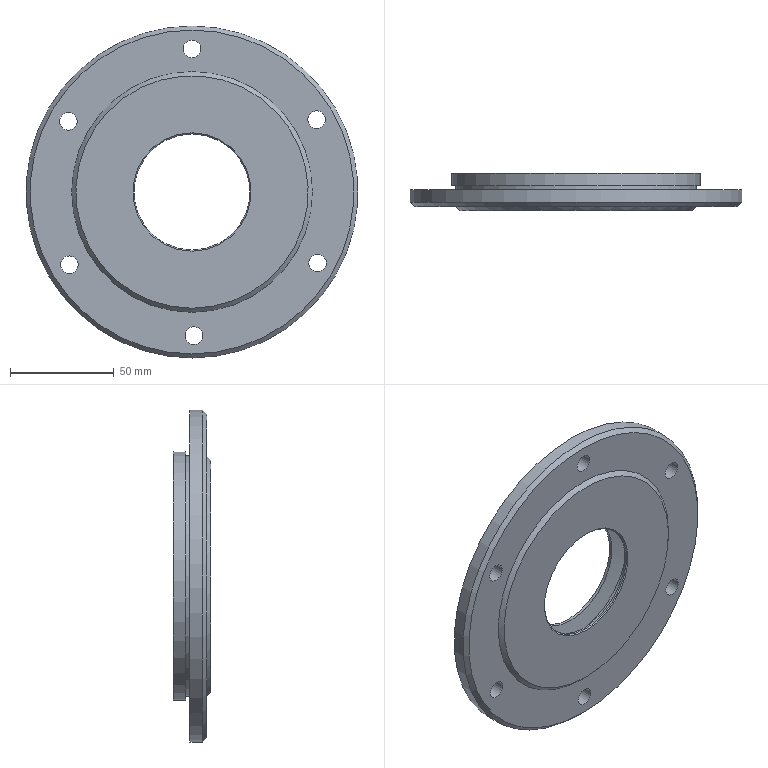Part | NX | features BREP 1, DATUM_CSYS 1 | 1 solid | 24 faces | box 160 x 18 x 160 mm | volume 177921 mm3 | cylinder 12 | plane 6 | cone 6 | commonest cylinder face diameters 8.5 x6 56 x2 74 x1 116 x1 120 x1 160 x1
STEP:
#1=CARTESIAN_POINT('',(419.528,84.,-38.494));
#2=VERTEX_POINT('',#1);
#3=CARTESIAN_POINT('',(419.528,84.,-34.244));
#4=DIRECTION('',(0.,-1.,0.));
#5=DIRECTION('',(0.,0.,-1.));
#6=AXIS2_PLACEMENT_3D('',#3,#4,#5);
#7=CIRCLE('',#6,4.25);
#8=EDGE_CURVE('',#2,#2,#7,.F.);
#9=ORIENTED_EDGE('',*,*,#8,.T.);
#10=EDGE_LOOP('',(#9));
#11=FACE_BOUND('',#10,.T.);
#12=CARTESIAN_POINT('',(359.92,84.,-73.44));
#13=VERTEX_POINT('',#12);
#14=CARTESIAN_POINT('',(359.92,84.,-69.19));
#15=DIRECTION('',(0.,-1.,0.));
#16=DIRECTION('',(0.,0.,-1.));
#17=AXIS2_PLACEMENT_3D('',#14,#15,#16);
#18=CIRCLE('',#17,4.25);
#19=EDGE_CURVE('',#13,#13,#18,.F.);
#20=ORIENTED_EDGE('',*,*,#19,.T.);
#21=EDGE_LOOP('',(#20));
#22=FACE_BOUND('',#21,.T.);
#23=CARTESIAN_POINT('',(299.852,84.,-39.291));
#24=VERTEX_POINT('',#23);
#25=CARTESIAN_POINT('',(299.852,84.,-35.041));
#26=DIRECTION('',(0.,-1.,0.));
#27=DIRECTION('',(0.,0.,-1.));
#28=AXIS2_PLACEMENT_3D('',#25,#26,#27);
#29=CIRCLE('',#28,4.25);
#30=EDGE_CURVE('',#24,#24,#29,.F.);
#31=ORIENTED_EDGE('',*,*,#30,.T.);
#32=EDGE_LOOP('',(#31));
#33=FACE_BOUND('',#32,.T.);
#34=CARTESIAN_POINT('',(299.392,84.,29.804));
#35=VERTEX_POINT('',#34);
#36=CARTESIAN_POINT('',(299.392,84.,34.054));
#37=DIRECTION('',(0.,-1.,0.));
#38=DIRECTION('',(0.,0.,-1.));
#39=AXIS2_PLACEMENT_3D('',#36,#37,#38);
#40=CIRCLE('',#39,4.25);
#41=EDGE_CURVE('',#35,#35,#40,.F.);
#42=ORIENTED_EDGE('',*,*,#41,.T.);
#43=EDGE_LOOP('',(#42));
#44=FACE_BOUND('',#43,.T.);
#45=CARTESIAN_POINT('',(359.,84.,64.75));
#46=VERTEX_POINT('',#45);
#47=CARTESIAN_POINT('',(359.,84.,69.));
#48=DIRECTION('',(0.,-1.,0.));
#49=DIRECTION('',(0.,0.,-1.));
#50=AXIS2_PLACEMENT_3D('',#47,#48,#49);
#51=CIRCLE('',#50,4.25);
#52=EDGE_CURVE('',#46,#46,#51,.F.);
#53=ORIENTED_EDGE('',*,*,#52,.T.);
#54=EDGE_LOOP('',(#53));
#55=FACE_BOUND('',#54,.T.);
#56=CARTESIAN_POINT('',(419.068,84.,30.601));
#57=VERTEX_POINT('',#56);
#58=CARTESIAN_POINT('',(419.068,84.,34.851));
#59=DIRECTION('',(0.,-1.,0.));
#60=DIRECTION('',(0.,0.,-1.));
#61=AXIS2_PLACEMENT_3D('',#58,#59,#60);
#62=CIRCLE('',#61,4.25);
#63=EDGE_CURVE('',#57,#57,#62,.F.);
#64=ORIENTED_EDGE('',*,*,#63,.T.);
#65=EDGE_LOOP('',(#64));
#66=FACE_BOUND('',#65,.T.);
#67=CARTESIAN_POINT('',(359.,84.,-78.));
#68=VERTEX_POINT('',#67);
#69=CARTESIAN_POINT('',(359.,84.,0.));
#70=DIRECTION('',(0.,-1.,0.));
#71=DIRECTION('',(0.,0.,-1.));
#72=AXIS2_PLACEMENT_3D('',#69,#70,#71);
#73=CIRCLE('',#72,78.);
#74=EDGE_CURVE('',#68,#68,#73,.T.);
#75=ORIENTED_EDGE('',*,*,#74,.T.);
#76=EDGE_LOOP('',(#75));
#77=FACE_BOUND('',#76,.T.);
#78=CARTESIAN_POINT('',(359.,84.,-58.));
#79=VERTEX_POINT('',#78);
#80=CARTESIAN_POINT('',(359.,84.,0.));
#81=DIRECTION('',(0.,-1.,0.));
#82=DIRECTION('',(0.,0.,-1.));
#83=AXIS2_PLACEMENT_3D('',#80,#81,#82);
#84=CIRCLE('',#83,58.);
#85=EDGE_CURVE('',#79,#79,#84,.T.);
#86=ORIENTED_EDGE('',*,*,#85,.F.);
#87=EDGE_LOOP('',(#86));
#88=FACE_BOUND('',#87,.T.);
#89=CARTESIAN_POINT('',(417.,84.,0.));
#90=DIRECTION('',(0.,-1.,0.));
#91=DIRECTION('',(0.,0.,-1.));
#92=AXIS2_PLACEMENT_3D('',#89,#90,#91);
#93=PLANE('',#92);
#94=ADVANCED_FACE('',(#11,#22,#33,#44,#55,#66,#77,#88),#93,.T.);
#95=CARTESIAN_POINT('',(359.,86.,-80.));
#96=VERTEX_POINT('',#95);
#97=CARTESIAN_POINT('',(359.,86.,0.));
#98=DIRECTION('',(0.,-1.,0.));
#99=DIRECTION('',(0.,0.,-1.));
#100=AXIS2_PLACEMENT_3D('',#97,#98,#99);
#101=CIRCLE('',#100,80.);
#102=EDGE_CURVE('',#96,#96,#101,.T.);
#103=ORIENTED_EDGE('',*,*,#102,.T.);
#104=EDGE_LOOP('',(#103));
#105=FACE_BOUND('',#104,.T.);
#106=ORIENTED_EDGE('',*,*,#74,.F.);
#107=EDGE_LOOP('',(#106));
#108=FACE_BOUND('',#107,.T.);
#109=CARTESIAN_POINT('',(359.,84.,0.));
#110=DIRECTION('',(0.,1.,0.));
#111=DIRECTION('',(0.,0.,1.));
#112=AXIS2_PLACEMENT_3D('',#109,#110,#111);
#113=CONICAL_SURFACE('',#112,78.,0.7854);
#114=ADVANCED_FACE('',(#105,#108),#113,.T.);
#115=CARTESIAN_POINT('',(359.,92.,-80.));
#116=VERTEX_POINT('',#115);
#117=CARTESIAN_POINT('',(359.,92.,0.));
#118=DIRECTION('',(0.,-1.,0.));
#119=DIRECTION('',(0.,0.,-1.));
#120=AXIS2_PLACEMENT_3D('',#117,#118,#119);
#121=CIRCLE('',#120,80.);
#122=EDGE_CURVE('',#116,#116,#121,.T.);
#123=ORIENTED_EDGE('',*,*,#122,.T.);
#124=EDGE_LOOP('',(#123));
#125=FACE_BOUND('',#124,.T.);
#126=ORIENTED_EDGE('',*,*,#102,.F.);
#127=EDGE_LOOP('',(#126));
#128=FACE_BOUND('',#127,.T.);
#129=CARTESIAN_POINT('',(359.,100.,0.));
#130=DIRECTION('',(0.,-1.,0.));
#131=DIRECTION('',(0.,0.,-1.));
#132=AXIS2_PLACEMENT_3D('',#129,#130,#131);
#133=CYLINDRICAL_SURFACE('',#132,80.);
#134=ADVANCED_FACE('',(#125,#128),#133,.T.);
#135=CARTESIAN_POINT('',(419.528,92.,-29.994));
#136=VERTEX_POINT('',#135);
#137=CARTESIAN_POINT('',(419.528,92.,-34.244));
#138=DIRECTION('',(0.,1.,0.));
#139=DIRECTION('',(0.,0.,1.));
#140=AXIS2_PLACEMENT_3D('',#137,#138,#139);
#141=CIRCLE('',#140,4.25);
#142=EDGE_CURVE('',#136,#136,#141,.F.);
#143=ORIENTED_EDGE('',*,*,#142,.T.);
#144=EDGE_LOOP('',(#143));
#145=FACE_BOUND('',#144,.T.);
#146=CARTESIAN_POINT('',(359.92,92.,-64.94));
#147=VERTEX_POINT('',#146);
#148=CARTESIAN_POINT('',(359.92,92.,-69.19));
#149=DIRECTION('',(0.,1.,0.));
#150=DIRECTION('',(0.,0.,1.));
#151=AXIS2_PLACEMENT_3D('',#148,#149,#150);
#152=CIRCLE('',#151,4.25);
#153=EDGE_CURVE('',#147,#147,#152,.F.);
#154=ORIENTED_EDGE('',*,*,#153,.T.);
#155=EDGE_LOOP('',(#154));
#156=FACE_BOUND('',#155,.T.);
#157=CARTESIAN_POINT('',(299.852,92.,-30.791));
#158=VERTEX_POINT('',#157);
#159=CARTESIAN_POINT('',(299.852,92.,-35.041));
#160=DIRECTION('',(0.,1.,0.));
#161=DIRECTION('',(0.,0.,1.));
#162=AXIS2_PLACEMENT_3D('',#159,#160,#161);
#163=CIRCLE('',#162,4.25);
#164=EDGE_CURVE('',#158,#158,#163,.F.);
#165=ORIENTED_EDGE('',*,*,#164,.T.);
#166=EDGE_LOOP('',(#165));
#167=FACE_BOUND('',#166,.T.);
#168=CARTESIAN_POINT('',(299.392,92.,38.304));
#169=VERTEX_POINT('',#168);
#170=CARTESIAN_POINT('',(299.392,92.,34.054));
#171=DIRECTION('',(0.,1.,0.));
#172=DIRECTION('',(0.,0.,1.));
#173=AXIS2_PLACEMENT_3D('',#170,#171,#172);
#174=CIRCLE('',#173,4.25);
#175=EDGE_CURVE('',#169,#169,#174,.F.);
#176=ORIENTED_EDGE('',*,*,#175,.T.);
#177=EDGE_LOOP('',(#176));
#178=FACE_BOUND('',#177,.T.);
#179=CARTESIAN_POINT('',(359.,92.,73.25));
#180=VERTEX_POINT('',#179);
#181=CARTESIAN_POINT('',(359.,92.,69.));
#182=DIRECTION('',(0.,1.,0.));
#183=DIRECTION('',(0.,0.,1.));
#184=AXIS2_PLACEMENT_3D('',#181,#182,#183);
#185=CIRCLE('',#184,4.25);
#186=EDGE_CURVE('',#180,#180,#185,.F.);
#187=ORIENTED_EDGE('',*,*,#186,.T.);
#188=EDGE_LOOP('',(#187));
#189=FACE_BOUND('',#188,.T.);
#190=CARTESIAN_POINT('',(419.068,92.,39.101));
#191=VERTEX_POINT('',#190);
#192=CARTESIAN_POINT('',(419.068,92.,34.851));
#193=DIRECTION('',(0.,1.,0.));
#194=DIRECTION('',(0.,0.,1.));
#195=AXIS2_PLACEMENT_3D('',#192,#193,#194);
#196=CIRCLE('',#195,4.25);
#197=EDGE_CURVE('',#191,#191,#196,.F.);
#198=ORIENTED_EDGE('',*,*,#197,.T.);
#199=EDGE_LOOP('',(#198));
#200=FACE_BOUND('',#199,.T.);
#201=CARTESIAN_POINT('',(359.,92.,-58.));
#202=VERTEX_POINT('',#201);
#203=CARTESIAN_POINT('',(359.,92.,0.));
#204=DIRECTION('',(0.,-1.,0.));
#205=DIRECTION('',(0.,0.,-1.));
#206=AXIS2_PLACEMENT_3D('',#203,#204,#205);
#207=CIRCLE('',#206,58.);
#208=EDGE_CURVE('',#202,#202,#207,.T.);
#209=ORIENTED_EDGE('',*,*,#208,.T.);
#210=EDGE_LOOP('',(#209));
#211=FACE_BOUND('',#210,.T.);
#212=ORIENTED_EDGE('',*,*,#122,.F.);
#213=EDGE_LOOP('',(#212));
#214=FACE_BOUND('',#213,.T.);
#215=CARTESIAN_POINT('',(439.,92.,0.));
#216=DIRECTION('',(0.,1.,0.));
#217=DIRECTION('',(0.,0.,1.));
#218=AXIS2_PLACEMENT_3D('',#215,#216,#217);
#219=PLANE('',#218);
#220=ADVANCED_FACE('',(#145,#156,#167,#178,#189,#200,#211,#214),#219,.T.);
#221=CARTESIAN_POINT('',(359.,94.,-58.));
#222=VERTEX_POINT('',#221);
#223=CARTESIAN_POINT('',(359.,94.,0.));
#224=DIRECTION('',(0.,-1.,0.));
#225=DIRECTION('',(0.,0.,-1.));
#226=AXIS2_PLACEMENT_3D('',#223,#224,#225);
#227=CIRCLE('',#226,58.);
#228=EDGE_CURVE('',#222,#222,#227,.T.);
#229=ORIENTED_EDGE('',*,*,#228,.T.);
#230=EDGE_LOOP('',(#229));
#231=FACE_BOUND('',#230,.T.);
#232=ORIENTED_EDGE('',*,*,#208,.F.);
#233=EDGE_LOOP('',(#232));
#234=FACE_BOUND('',#233,.T.);
#235=CARTESIAN_POINT('',(359.,100.,0.));
#236=DIRECTION('',(0.,-1.,0.));
#237=DIRECTION('',(0.,0.,-1.));
#238=AXIS2_PLACEMENT_3D('',#235,#236,#237);
#239=CYLINDRICAL_SURFACE('',#238,58.);
#240=ADVANCED_FACE('',(#231,#234),#239,.T.);
#241=CARTESIAN_POINT('',(359.,94.,-60.));
#242=VERTEX_POINT('',#241);
#243=CARTESIAN_POINT('',(359.,94.,0.));
#244=DIRECTION('',(0.,-1.,0.));
#245=DIRECTION('',(0.,0.,-1.));
#246=AXIS2_PLACEMENT_3D('',#243,#244,#245);
#247=CIRCLE('',#246,60.);
#248=EDGE_CURVE('',#242,#242,#247,.T.);
#249=ORIENTED_EDGE('',*,*,#248,.T.);
#250=EDGE_LOOP('',(#249));
#251=FACE_BOUND('',#250,.T.);
#252=ORIENTED_EDGE('',*,*,#228,.F.);
#253=EDGE_LOOP('',(#252));
#254=FACE_BOUND('',#253,.T.);
#255=CARTESIAN_POINT('',(417.,94.,0.));
#256=DIRECTION('',(0.,-1.,0.));
#257=DIRECTION('',(0.,0.,-1.));
#258=AXIS2_PLACEMENT_3D('',#255,#256,#257);
#259=PLANE('',#258);
#260=ADVANCED_FACE('',(#251,#254),#259,.T.);
#261=CARTESIAN_POINT('',(359.,100.,-60.));
#262=VERTEX_POINT('',#261);
#263=CARTESIAN_POINT('',(359.,100.,0.));
#264=DIRECTION('',(0.,-1.,0.));
#265=DIRECTION('',(0.,0.,-1.));
#266=AXIS2_PLACEMENT_3D('',#263,#264,#265);
#267=CIRCLE('',#266,60.);
#268=EDGE_CURVE('',#262,#262,#267,.T.);
#269=ORIENTED_EDGE('',*,*,#268,.T.);
#270=EDGE_LOOP('',(#269));
#271=FACE_BOUND('',#270,.T.);
#272=ORIENTED_EDGE('',*,*,#248,.F.);
#273=EDGE_LOOP('',(#272));
#274=FACE_BOUND('',#273,.T.);
#275=CARTESIAN_POINT('',(359.,100.,0.));
#276=DIRECTION('',(0.,-1.,0.));
#277=DIRECTION('',(0.,0.,-1.));
#278=AXIS2_PLACEMENT_3D('',#275,#276,#277);
#279=CYLINDRICAL_SURFACE('',#278,60.);
#280=ADVANCED_FACE('',(#271,#274),#279,.T.);
#281=CARTESIAN_POINT('',(359.,100.,-50.));
#282=VERTEX_POINT('',#281);
#283=CARTESIAN_POINT('',(359.,100.,0.));
#284=DIRECTION('',(0.,-1.,0.));
#285=DIRECTION('',(0.,0.,-1.));
#286=AXIS2_PLACEMENT_3D('',#283,#284,#285);
#287=CIRCLE('',#286,50.);
#288=EDGE_CURVE('',#282,#282,#287,.T.);
#289=ORIENTED_EDGE('',*,*,#288,.T.);
#290=EDGE_LOOP('',(#289));
#291=FACE_BOUND('',#290,.T.);
#292=ORIENTED_EDGE('',*,*,#268,.F.);
#293=EDGE_LOOP('',(#292));
#294=FACE_BOUND('',#293,.T.);
#295=CARTESIAN_POINT('',(419.,100.,0.));
#296=DIRECTION('',(0.,1.,0.));
#297=DIRECTION('',(0.,0.,1.));
#298=AXIS2_PLACEMENT_3D('',#295,#296,#297);
#299=PLANE('',#298);
#300=ADVANCED_FACE('',(#291,#294),#299,.T.);
#301=CARTESIAN_POINT('',(359.,94.,-47.816));
#302=VERTEX_POINT('',#301);
#303=CARTESIAN_POINT('',(359.,94.,0.));
#304=DIRECTION('',(0.,-1.,0.));
#305=DIRECTION('',(0.,0.,-1.));
#306=AXIS2_PLACEMENT_3D('',#303,#304,#305);
#307=CIRCLE('',#306,47.816);
#308=EDGE_CURVE('',#302,#302,#307,.T.);
#309=ORIENTED_EDGE('',*,*,#308,.T.);
#310=EDGE_LOOP('',(#309));
#311=FACE_BOUND('',#310,.T.);
#312=ORIENTED_EDGE('',*,*,#288,.F.);
#313=EDGE_LOOP('',(#312));
#314=FACE_BOUND('',#313,.T.);
#315=CARTESIAN_POINT('',(359.,100.,0.));
#316=DIRECTION('',(0.,1.,0.));
#317=DIRECTION('',(0.,0.,1.));
#318=AXIS2_PLACEMENT_3D('',#315,#316,#317);
#319=CONICAL_SURFACE('',#318,50.,0.3491);
#320=ADVANCED_FACE('',(#311,#314),#319,.F.);
#321=CARTESIAN_POINT('',(359.,94.,-28.));
#322=VERTEX_POINT('',#321);
#323=CARTESIAN_POINT('',(359.,94.,0.));
#324=DIRECTION('',(0.,-1.,0.));
#325=DIRECTION('',(0.,0.,-1.));
#326=AXIS2_PLACEMENT_3D('',#323,#324,#325);
#327=CIRCLE('',#326,28.);
#328=EDGE_CURVE('',#322,#322,#327,.T.);
#329=ORIENTED_EDGE('',*,*,#328,.T.);
#330=EDGE_LOOP('',(#329));
#331=FACE_BOUND('',#330,.T.);
#332=ORIENTED_EDGE('',*,*,#308,.F.);
#333=EDGE_LOOP('',(#332));
#334=FACE_BOUND('',#333,.T.);
#335=CARTESIAN_POINT('',(406.816,94.,0.));
#336=DIRECTION('',(0.,1.,0.));
#337=DIRECTION('',(0.,0.,1.));
#338=AXIS2_PLACEMENT_3D('',#335,#336,#337);
#339=PLANE('',#338);
#340=ADVANCED_FACE('',(#331,#334),#339,.T.);
#341=CARTESIAN_POINT('',(359.,92.5,-28.));
#342=VERTEX_POINT('',#341);
#343=CARTESIAN_POINT('',(359.,92.5,0.));
#344=DIRECTION('',(0.,-1.,0.));
#345=DIRECTION('',(0.,0.,-1.));
#346=AXIS2_PLACEMENT_3D('',#343,#344,#345);
#347=CIRCLE('',#346,28.);
#348=EDGE_CURVE('',#342,#342,#347,.T.);
#349=ORIENTED_EDGE('',*,*,#348,.T.);
#350=EDGE_LOOP('',(#349));
#351=FACE_BOUND('',#350,.T.);
#352=ORIENTED_EDGE('',*,*,#328,.F.);
#353=EDGE_LOOP('',(#352));
#354=FACE_BOUND('',#353,.T.);
#355=CARTESIAN_POINT('',(359.,100.,0.));
#356=DIRECTION('',(0.,-1.,0.));
#357=DIRECTION('',(0.,0.,-1.));
#358=AXIS2_PLACEMENT_3D('',#355,#356,#357);
#359=CYLINDRICAL_SURFACE('',#358,28.);
#360=ADVANCED_FACE('',(#351,#354),#359,.F.);
#361=CARTESIAN_POINT('',(359.,91.15,-37.));
#362=VERTEX_POINT('',#361);
#363=CARTESIAN_POINT('',(359.,91.15,0.));
#364=DIRECTION('',(0.,-1.,0.));
#365=DIRECTION('',(0.,0.,-1.));
#366=AXIS2_PLACEMENT_3D('',#363,#364,#365);
#367=CIRCLE('',#366,37.);
#368=EDGE_CURVE('',#362,#362,#367,.T.);
#369=ORIENTED_EDGE('',*,*,#368,.T.);
#370=EDGE_LOOP('',(#369));
#371=FACE_BOUND('',#370,.T.);
#372=ORIENTED_EDGE('',*,*,#348,.F.);
#373=EDGE_LOOP('',(#372));
#374=FACE_BOUND('',#373,.T.);
#375=CARTESIAN_POINT('',(359.,92.5,0.));
#376=DIRECTION('',(0.,-1.,0.));
#377=DIRECTION('',(0.,0.,-1.));
#378=AXIS2_PLACEMENT_3D('',#375,#376,#377);
#379=CONICAL_SURFACE('',#378,28.,1.422);
#380=ADVANCED_FACE('',(#371,#374),#379,.F.);
#381=CARTESIAN_POINT('',(359.,84.85,-37.));
#382=VERTEX_POINT('',#381);
#383=CARTESIAN_POINT('',(359.,84.85,0.));
#384=DIRECTION('',(0.,-1.,0.));
#385=DIRECTION('',(0.,0.,-1.));
#386=AXIS2_PLACEMENT_3D('',#383,#384,#385);
#387=CIRCLE('',#386,37.);
#388=EDGE_CURVE('',#382,#382,#387,.T.);
#389=ORIENTED_EDGE('',*,*,#388,.T.);
#390=EDGE_LOOP('',(#389));
#391=FACE_BOUND('',#390,.T.);
#392=ORIENTED_EDGE('',*,*,#368,.F.);
#393=EDGE_LOOP('',(#392));
#394=FACE_BOUND('',#393,.T.);
#395=CARTESIAN_POINT('',(359.,100.,0.));
#396=DIRECTION('',(0.,-1.,0.));
#397=DIRECTION('',(0.,0.,-1.));
#398=AXIS2_PLACEMENT_3D('',#395,#396,#397);
#399=CYLINDRICAL_SURFACE('',#398,37.);
#400=ADVANCED_FACE('',(#391,#394),#399,.F.);
#401=CARTESIAN_POINT('',(359.,83.5,-28.));
#402=VERTEX_POINT('',#401);
#403=CARTESIAN_POINT('',(359.,83.5,0.));
#404=DIRECTION('',(0.,-1.,0.));
#405=DIRECTION('',(0.,0.,-1.));
#406=AXIS2_PLACEMENT_3D('',#403,#404,#405);
#407=CIRCLE('',#406,28.);
#408=EDGE_CURVE('',#402,#402,#407,.T.);
#409=ORIENTED_EDGE('',*,*,#408,.T.);
#410=EDGE_LOOP('',(#409));
#411=FACE_BOUND('',#410,.T.);
#412=ORIENTED_EDGE('',*,*,#388,.F.);
#413=EDGE_LOOP('',(#412));
#414=FACE_BOUND('',#413,.T.);
#415=CARTESIAN_POINT('',(359.,84.85,0.));
#416=DIRECTION('',(0.,1.,0.));
#417=DIRECTION('',(0.,0.,1.));
#418=AXIS2_PLACEMENT_3D('',#415,#416,#417);
#419=CONICAL_SURFACE('',#418,37.,1.422);
#420=ADVANCED_FACE('',(#411,#414),#419,.F.);
#421=CARTESIAN_POINT('',(359.,82.5,-28.));
#422=VERTEX_POINT('',#421);
#423=CARTESIAN_POINT('',(359.,82.5,0.));
#424=DIRECTION('',(0.,-1.,0.));
#425=DIRECTION('',(0.,0.,-1.));
#426=AXIS2_PLACEMENT_3D('',#423,#424,#425);
#427=CIRCLE('',#426,28.);
#428=EDGE_CURVE('',#422,#422,#427,.T.);
#429=ORIENTED_EDGE('',*,*,#428,.T.);
#430=EDGE_LOOP('',(#429));
#431=FACE_BOUND('',#430,.T.);
#432=ORIENTED_EDGE('',*,*,#408,.F.);
#433=EDGE_LOOP('',(#432));
#434=FACE_BOUND('',#433,.T.);
#435=CARTESIAN_POINT('',(359.,100.,0.));
#436=DIRECTION('',(0.,-1.,0.));
#437=DIRECTION('',(0.,0.,-1.));
#438=AXIS2_PLACEMENT_3D('',#435,#436,#437);
#439=CYLINDRICAL_SURFACE('',#438,28.);
#440=ADVANCED_FACE('',(#431,#434),#439,.F.);
#441=CARTESIAN_POINT('',(359.,82.,-28.5));
#442=VERTEX_POINT('',#441);
#443=CARTESIAN_POINT('',(359.,82.,0.));
#444=DIRECTION('',(0.,-1.,0.));
#445=DIRECTION('',(0.,0.,-1.));
#446=AXIS2_PLACEMENT_3D('',#443,#444,#445);
#447=CIRCLE('',#446,28.5);
#448=EDGE_CURVE('',#442,#442,#447,.T.);
#449=ORIENTED_EDGE('',*,*,#448,.T.);
#450=EDGE_LOOP('',(#449));
#451=FACE_BOUND('',#450,.T.);
#452=ORIENTED_EDGE('',*,*,#428,.F.);
#453=EDGE_LOOP('',(#452));
#454=FACE_BOUND('',#453,.T.);
#455=CARTESIAN_POINT('',(359.,82.5,0.));
#456=DIRECTION('',(0.,-1.,0.));
#457=DIRECTION('',(0.,0.,-1.));
#458=AXIS2_PLACEMENT_3D('',#455,#456,#457);
#459=CONICAL_SURFACE('',#458,28.,0.7854);
#460=ADVANCED_FACE('',(#451,#454),#459,.F.);
#461=CARTESIAN_POINT('',(359.,82.,-56.));
#462=VERTEX_POINT('',#461);
#463=CARTESIAN_POINT('',(359.,82.,0.));
#464=DIRECTION('',(0.,-1.,0.));
#465=DIRECTION('',(0.,0.,-1.));
#466=AXIS2_PLACEMENT_3D('',#463,#464,#465);
#467=CIRCLE('',#466,56.);
#468=EDGE_CURVE('',#462,#462,#467,.T.);
#469=ORIENTED_EDGE('',*,*,#468,.T.);
#470=EDGE_LOOP('',(#469));
#471=FACE_BOUND('',#470,.T.);
#472=ORIENTED_EDGE('',*,*,#448,.F.);
#473=EDGE_LOOP('',(#472));
#474=FACE_BOUND('',#473,.T.);
#475=CARTESIAN_POINT('',(387.5,82.,0.));
#476=DIRECTION('',(0.,-1.,0.));
#477=DIRECTION('',(0.,0.,-1.));
#478=AXIS2_PLACEMENT_3D('',#475,#476,#477);
#479=PLANE('',#478);
#480=ADVANCED_FACE('',(#471,#474),#479,.T.);
#481=ORIENTED_EDGE('',*,*,#85,.T.);
#482=EDGE_LOOP('',(#481));
#483=FACE_BOUND('',#482,.T.);
#484=ORIENTED_EDGE('',*,*,#468,.F.);
#485=EDGE_LOOP('',(#484));
#486=FACE_BOUND('',#485,.T.);
#487=CARTESIAN_POINT('',(359.,82.,0.));
#488=DIRECTION('',(0.,1.,0.));
#489=DIRECTION('',(0.,0.,1.));
#490=AXIS2_PLACEMENT_3D('',#487,#488,#489);
#491=CONICAL_SURFACE('',#490,56.,0.7854);
#492=ADVANCED_FACE('',(#483,#486),#491,.T.);
#493=ORIENTED_EDGE('',*,*,#63,.F.);
#494=EDGE_LOOP('',(#493));
#495=FACE_BOUND('',#494,.T.);
#496=ORIENTED_EDGE('',*,*,#197,.F.);
#497=EDGE_LOOP('',(#496));
#498=FACE_BOUND('',#497,.T.);
#499=CARTESIAN_POINT('',(419.068,36.,34.851));
#500=DIRECTION('',(0.,1.,0.));
#501=DIRECTION('',(0.,0.,1.));
#502=AXIS2_PLACEMENT_3D('',#499,#500,#501);
#503=CYLINDRICAL_SURFACE('',#502,4.25);
#504=ADVANCED_FACE('',(#495,#498),#503,.F.);
#505=ORIENTED_EDGE('',*,*,#52,.F.);
#506=EDGE_LOOP('',(#505));
#507=FACE_BOUND('',#506,.T.);
#508=ORIENTED_EDGE('',*,*,#186,.F.);
#509=EDGE_LOOP('',(#508));
#510=FACE_BOUND('',#509,.T.);
#511=CARTESIAN_POINT('',(359.,36.,69.));
#512=DIRECTION('',(0.,1.,0.));
#513=DIRECTION('',(0.,0.,1.));
#514=AXIS2_PLACEMENT_3D('',#511,#512,#513);
#515=CYLINDRICAL_SURFACE('',#514,4.25);
#516=ADVANCED_FACE('',(#507,#510),#515,.F.);
#517=ORIENTED_EDGE('',*,*,#41,.F.);
#518=EDGE_LOOP('',(#517));
#519=FACE_BOUND('',#518,.T.);
#520=ORIENTED_EDGE('',*,*,#175,.F.);
#521=EDGE_LOOP('',(#520));
#522=FACE_BOUND('',#521,.T.);
#523=CARTESIAN_POINT('',(299.392,36.,34.054));
#524=DIRECTION('',(0.,1.,0.));
#525=DIRECTION('',(0.,0.,1.));
#526=AXIS2_PLACEMENT_3D('',#523,#524,#525);
#527=CYLINDRICAL_SURFACE('',#526,4.25);
#528=ADVANCED_FACE('',(#519,#522),#527,.F.);
#529=ORIENTED_EDGE('',*,*,#30,.F.);
#530=EDGE_LOOP('',(#529));
#531=FACE_BOUND('',#530,.T.);
#532=ORIENTED_EDGE('',*,*,#164,.F.);
#533=EDGE_LOOP('',(#532));
#534=FACE_BOUND('',#533,.T.);
#535=CARTESIAN_POINT('',(299.852,36.,-35.041));
#536=DIRECTION('',(0.,1.,0.));
#537=DIRECTION('',(0.,0.,1.));
#538=AXIS2_PLACEMENT_3D('',#535,#536,#537);
#539=CYLINDRICAL_SURFACE('',#538,4.25);
#540=ADVANCED_FACE('',(#531,#534),#539,.F.);
#541=ORIENTED_EDGE('',*,*,#19,.F.);
#542=EDGE_LOOP('',(#541));
#543=FACE_BOUND('',#542,.T.);
#544=ORIENTED_EDGE('',*,*,#153,.F.);
#545=EDGE_LOOP('',(#544));
#546=FACE_BOUND('',#545,.T.);
#547=CARTESIAN_POINT('',(359.92,36.,-69.19));
#548=DIRECTION('',(0.,1.,0.));
#549=DIRECTION('',(0.,0.,1.));
#550=AXIS2_PLACEMENT_3D('',#547,#548,#549);
#551=CYLINDRICAL_SURFACE('',#550,4.25);
#552=ADVANCED_FACE('',(#543,#546),#551,.F.);
#553=ORIENTED_EDGE('',*,*,#8,.F.);
#554=EDGE_LOOP('',(#553));
#555=FACE_BOUND('',#554,.T.);
#556=ORIENTED_EDGE('',*,*,#142,.F.);
#557=EDGE_LOOP('',(#556));
#558=FACE_BOUND('',#557,.T.);
#559=CARTESIAN_POINT('',(419.528,36.,-34.244));
#560=DIRECTION('',(0.,1.,0.));
#561=DIRECTION('',(0.,0.,1.));
#562=AXIS2_PLACEMENT_3D('',#559,#560,#561);
#563=CYLINDRICAL_SURFACE('',#562,4.25);
#564=ADVANCED_FACE('',(#555,#558),#563,.F.);
#565=CLOSED_SHELL('',(#94,#114,#134,#220,#240,#260,#280,#300,#320,#340,#360,#380,#400,#420,#440,#460,#480,#492,#504,#516,#528,#540,#552,#564));
#566=MANIFOLD_SOLID_BREP('',#565);
#567=(LENGTH_UNIT()NAMED_UNIT(*)SI_UNIT(.MILLI.,.METRE.));
#568=UNCERTAINTY_MEASURE_WITH_UNIT(LENGTH_MEASURE(0.00001),#567,'','');
#569=(NAMED_UNIT(*)PLANE_ANGLE_UNIT()SI_UNIT($,.RADIAN.));
#570=(NAMED_UNIT(*)SI_UNIT($,.STERADIAN.)SOLID_ANGLE_UNIT());
#571=(GEOMETRIC_REPRESENTATION_CONTEXT(3)GLOBAL_UNCERTAINTY_ASSIGNED_CONTEXT((#568))GLOBAL_UNIT_ASSIGNED_CONTEXT((#567,#569,#570))REPRESENTATION_CONTEXT('',''));
#572=ADVANCED_BREP_SHAPE_REPRESENTATION('',(#566),#571);